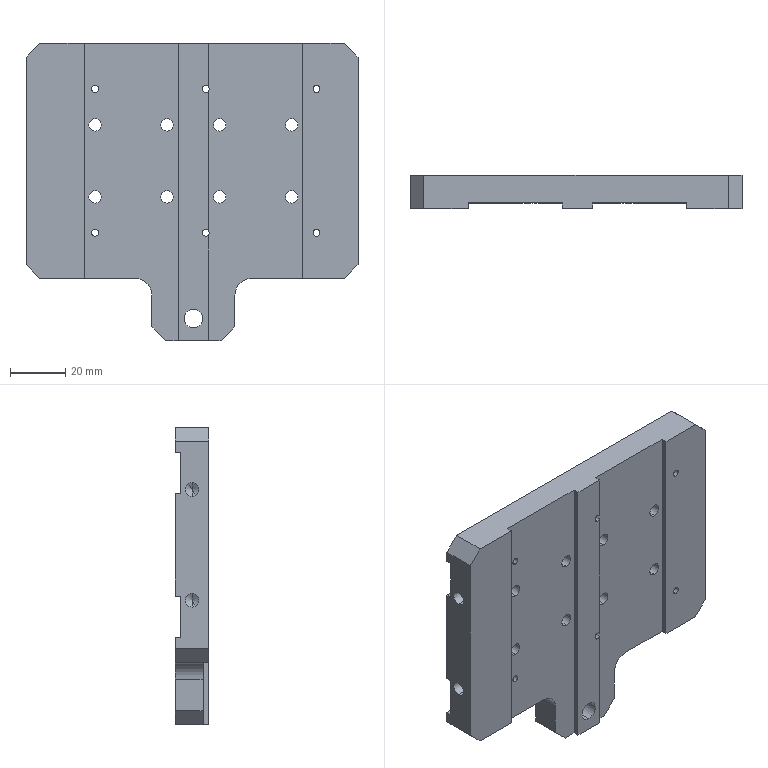Part | STEP file | PN_0019 | 1 solid | 98 faces | box 120 x 12 x 107.5 mm | volume 106389 mm3 | cylinder 52 | plane 42 | cone 4 | commonest cylinder face diameters 4.5 x16 8 x16 2.5 x12 5 x4 6.8 x2 12 x2